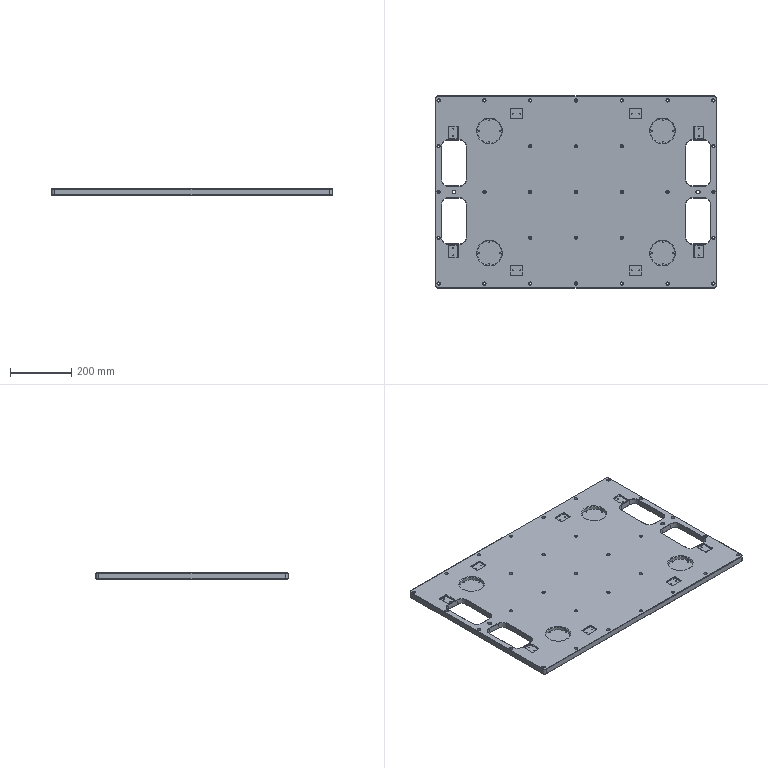Part | STEP file | TJ-DHQM-004-007 | 1 solid | 518 faces | box 920 x 630 x 20 mm | volume 10320412 mm3 | cylinder 253 | plane 175 | cone 90 | commonest cylinder face diameters 3.3 x64 6.6 x62 11 x62 5 x32 40 x16 80 x8